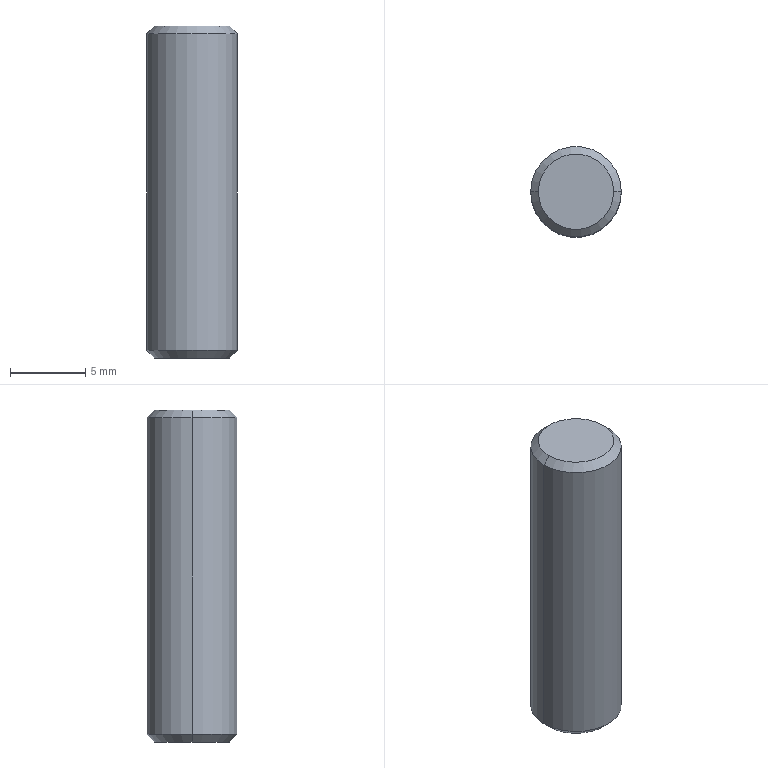Part | STEP file | 03-18 guide post A | 1 solid | 12 faces | box 6 x 6 x 22 mm | volume 567.268 mm3 | cone 6 | cylinder 4 | plane 2 | commonest cylinder face diameters 2.5 x2 6 x2
STEP:
#1=CARTESIAN_POINT('',(1.25,0.,10.));
#2=VERTEX_POINT('',#1);
#3=CARTESIAN_POINT('',(-1.25,0.,10.));
#4=VERTEX_POINT('',#3);
#5=CARTESIAN_POINT('',(0.,0.,10.));
#6=DIRECTION('',(0.,0.,-1.));
#7=DIRECTION('',(-1.,0.,0.));
#8=AXIS2_PLACEMENT_3D('',#5,#6,#7);
#9=CIRCLE('',#8,1.25);
#10=EDGE_CURVE('',#2,#4,#9,.T.);
#11=ORIENTED_EDGE('',*,*,#10,.F.);
#12=CARTESIAN_POINT('',(1.25,0.,0.));
#13=VERTEX_POINT('',#12);
#14=CARTESIAN_POINT('',(1.25,0.,0.));
#15=DIRECTION('',(0.,0.,-1.));
#16=VECTOR('',#15,1000.);
#17=LINE('',#14,#16);
#18=EDGE_CURVE('',#2,#13,#17,.T.);
#19=ORIENTED_EDGE('',*,*,#18,.T.);
#20=CARTESIAN_POINT('',(-1.25,0.,0.));
#21=VERTEX_POINT('',#20);
#22=CARTESIAN_POINT('',(0.,0.,0.));
#23=DIRECTION('',(0.,0.,-1.));
#24=DIRECTION('',(-1.,0.,0.));
#25=AXIS2_PLACEMENT_3D('',#22,#23,#24);
#26=CIRCLE('',#25,1.25);
#27=EDGE_CURVE('',#13,#21,#26,.T.);
#28=ORIENTED_EDGE('',*,*,#27,.T.);
#29=CARTESIAN_POINT('',(-1.25,0.,0.));
#30=DIRECTION('',(0.,0.,-1.));
#31=VECTOR('',#30,1000.);
#32=LINE('',#29,#31);
#33=EDGE_CURVE('',#4,#21,#32,.T.);
#34=ORIENTED_EDGE('',*,*,#33,.F.);
#35=EDGE_LOOP('',(#11,#19,#28,#34));
#36=FACE_OUTER_BOUND('',#35,.T.);
#37=CARTESIAN_POINT('',(0.,0.,0.));
#38=DIRECTION('',(0.,0.,-1.));
#39=DIRECTION('',(-1.,0.,0.));
#40=AXIS2_PLACEMENT_3D('',#37,#38,#39);
#41=CYLINDRICAL_SURFACE('',#40,1.25);
#42=ADVANCED_FACE('',(#36),#41,.F.);
#43=CARTESIAN_POINT('',(0.,0.,10.751));
#44=VERTEX_POINT('',#43);
#45=CARTESIAN_POINT('',(-1.25,0.,10.));
#46=DIRECTION('',(-0.8572,0.,-0.515));
#47=VECTOR('',#46,1000.);
#48=LINE('',#45,#47);
#49=EDGE_CURVE('',#44,#4,#48,.T.);
#50=ORIENTED_EDGE('',*,*,#49,.F.);
#51=CARTESIAN_POINT('',(1.25,0.,10.));
#52=DIRECTION('',(0.8572,0.,-0.515));
#53=VECTOR('',#52,1000.);
#54=LINE('',#51,#53);
#55=EDGE_CURVE('',#44,#2,#54,.T.);
#56=ORIENTED_EDGE('',*,*,#55,.T.);
#57=ORIENTED_EDGE('',*,*,#10,.T.);
#58=EDGE_LOOP('',(#50,#56,#57));
#59=FACE_OUTER_BOUND('',#58,.T.);
#60=CARTESIAN_POINT('',(0.,0.,10.));
#61=DIRECTION('',(0.,0.,-1.));
#62=DIRECTION('',(-1.,0.,0.));
#63=AXIS2_PLACEMENT_3D('',#60,#61,#62);
#64=CONICAL_SURFACE('',#63,1.25,1.03);
#65=ADVANCED_FACE('',(#59),#64,.F.);
#66=CARTESIAN_POINT('',(-2.5,0.,0.));
#67=VERTEX_POINT('',#66);
#68=CARTESIAN_POINT('',(2.5,0.,0.));
#69=VERTEX_POINT('',#68);
#70=CARTESIAN_POINT('',(0.,0.,0.));
#71=DIRECTION('',(0.,0.,-1.));
#72=DIRECTION('',(1.,0.,0.));
#73=AXIS2_PLACEMENT_3D('',#70,#71,#72);
#74=CIRCLE('',#73,2.5);
#75=EDGE_CURVE('',#67,#69,#74,.T.);
#76=ORIENTED_EDGE('',*,*,#75,.F.);
#77=CARTESIAN_POINT('',(-3.,0.,0.5));
#78=VERTEX_POINT('',#77);
#79=CARTESIAN_POINT('',(-3.,0.,0.5));
#80=DIRECTION('',(-0.7071,0.,0.7071));
#81=VECTOR('',#80,1000.);
#82=LINE('',#79,#81);
#83=EDGE_CURVE('',#67,#78,#82,.T.);
#84=ORIENTED_EDGE('',*,*,#83,.T.);
#85=CARTESIAN_POINT('',(3.,0.,0.5));
#86=VERTEX_POINT('',#85);
#87=CARTESIAN_POINT('',(0.,0.,0.5));
#88=DIRECTION('',(0.,0.,1.));
#89=DIRECTION('',(1.,0.,0.));
#90=AXIS2_PLACEMENT_3D('',#87,#88,#89);
#91=CIRCLE('',#90,3.);
#92=EDGE_CURVE('',#86,#78,#91,.T.);
#93=ORIENTED_EDGE('',*,*,#92,.F.);
#94=CARTESIAN_POINT('',(3.,0.,0.5));
#95=DIRECTION('',(0.7071,0.,0.7071));
#96=VECTOR('',#95,1000.);
#97=LINE('',#94,#96);
#98=EDGE_CURVE('',#69,#86,#97,.T.);
#99=ORIENTED_EDGE('',*,*,#98,.F.);
#100=EDGE_LOOP('',(#76,#84,#93,#99));
#101=FACE_OUTER_BOUND('',#100,.T.);
#102=CARTESIAN_POINT('',(0.,0.,0.5));
#103=DIRECTION('',(0.,0.,1.));
#104=DIRECTION('',(1.,0.,0.));
#105=AXIS2_PLACEMENT_3D('',#102,#103,#104);
#106=CONICAL_SURFACE('',#105,3.,0.7854);
#107=ADVANCED_FACE('',(#101),#106,.T.);
#108=CARTESIAN_POINT('',(2.5,0.,22.));
#109=VERTEX_POINT('',#108);
#110=CARTESIAN_POINT('',(-2.5,0.,22.));
#111=VERTEX_POINT('',#110);
#112=CARTESIAN_POINT('',(0.,0.,22.));
#113=DIRECTION('',(0.,0.,1.));
#114=DIRECTION('',(1.,0.,0.));
#115=AXIS2_PLACEMENT_3D('',#112,#113,#114);
#116=CIRCLE('',#115,2.5);
#117=EDGE_CURVE('',#109,#111,#116,.T.);
#118=ORIENTED_EDGE('',*,*,#117,.F.);
#119=CARTESIAN_POINT('',(3.,0.,21.5));
#120=VERTEX_POINT('',#119);
#121=CARTESIAN_POINT('',(2.5,0.,22.));
#122=DIRECTION('',(0.7071,0.,-0.7071));
#123=VECTOR('',#122,1000.);
#124=LINE('',#121,#123);
#125=EDGE_CURVE('',#109,#120,#124,.T.);
#126=ORIENTED_EDGE('',*,*,#125,.T.);
#127=CARTESIAN_POINT('',(-3.,0.,21.5));
#128=VERTEX_POINT('',#127);
#129=CARTESIAN_POINT('',(0.,0.,21.5));
#130=DIRECTION('',(0.,0.,-1.));
#131=DIRECTION('',(1.,0.,0.));
#132=AXIS2_PLACEMENT_3D('',#129,#130,#131);
#133=CIRCLE('',#132,3.);
#134=EDGE_CURVE('',#128,#120,#133,.T.);
#135=ORIENTED_EDGE('',*,*,#134,.F.);
#136=CARTESIAN_POINT('',(-2.5,0.,22.));
#137=DIRECTION('',(-0.7071,0.,-0.7071));
#138=VECTOR('',#137,1000.);
#139=LINE('',#136,#138);
#140=EDGE_CURVE('',#111,#128,#139,.T.);
#141=ORIENTED_EDGE('',*,*,#140,.F.);
#142=EDGE_LOOP('',(#118,#126,#135,#141));
#143=FACE_OUTER_BOUND('',#142,.T.);
#144=CARTESIAN_POINT('',(0.,0.,22.));
#145=DIRECTION('',(0.,0.,-1.));
#146=DIRECTION('',(-1.,0.,0.));
#147=AXIS2_PLACEMENT_3D('',#144,#145,#146);
#148=CONICAL_SURFACE('',#147,2.5,0.7854);
#149=ADVANCED_FACE('',(#143),#148,.T.);
#150=ORIENTED_EDGE('',*,*,#134,.T.);
#151=CARTESIAN_POINT('',(3.,0.,22.));
#152=DIRECTION('',(0.,0.,-1.));
#153=VECTOR('',#152,1000.);
#154=LINE('',#151,#153);
#155=EDGE_CURVE('',#120,#86,#154,.T.);
#156=ORIENTED_EDGE('',*,*,#155,.T.);
#157=ORIENTED_EDGE('',*,*,#92,.T.);
#158=CARTESIAN_POINT('',(-3.,0.,22.));
#159=DIRECTION('',(0.,0.,-1.));
#160=VECTOR('',#159,1000.);
#161=LINE('',#158,#160);
#162=EDGE_CURVE('',#128,#78,#161,.T.);
#163=ORIENTED_EDGE('',*,*,#162,.F.);
#164=EDGE_LOOP('',(#150,#156,#157,#163));
#165=FACE_OUTER_BOUND('',#164,.T.);
#166=CARTESIAN_POINT('',(0.,0.,22.));
#167=DIRECTION('',(0.,0.,-1.));
#168=DIRECTION('',(-1.,0.,0.));
#169=AXIS2_PLACEMENT_3D('',#166,#167,#168);
#170=CYLINDRICAL_SURFACE('',#169,3.);
#171=ADVANCED_FACE('',(#165),#170,.T.);
#172=ORIENTED_EDGE('',*,*,#155,.F.);
#173=CARTESIAN_POINT('',(0.,0.,21.5));
#174=DIRECTION('',(0.,0.,-1.));
#175=DIRECTION('',(1.,0.,0.));
#176=AXIS2_PLACEMENT_3D('',#173,#174,#175);
#177=CIRCLE('',#176,3.);
#178=EDGE_CURVE('',#120,#128,#177,.T.);
#179=ORIENTED_EDGE('',*,*,#178,.T.);
#180=ORIENTED_EDGE('',*,*,#162,.T.);
#181=CARTESIAN_POINT('',(0.,0.,0.5));
#182=DIRECTION('',(0.,0.,1.));
#183=DIRECTION('',(1.,0.,0.));
#184=AXIS2_PLACEMENT_3D('',#181,#182,#183);
#185=CIRCLE('',#184,3.);
#186=EDGE_CURVE('',#78,#86,#185,.T.);
#187=ORIENTED_EDGE('',*,*,#186,.T.);
#188=EDGE_LOOP('',(#172,#179,#180,#187));
#189=FACE_OUTER_BOUND('',#188,.T.);
#190=CARTESIAN_POINT('',(0.,0.,22.));
#191=DIRECTION('',(0.,0.,-1.));
#192=DIRECTION('',(-1.,0.,0.));
#193=AXIS2_PLACEMENT_3D('',#190,#191,#192);
#194=CYLINDRICAL_SURFACE('',#193,3.);
#195=ADVANCED_FACE('',(#189),#194,.T.);
#196=CARTESIAN_POINT('',(0.,0.,22.));
#197=DIRECTION('',(0.,0.,1.));
#198=DIRECTION('',(1.,0.,0.));
#199=AXIS2_PLACEMENT_3D('',#196,#197,#198);
#200=CIRCLE('',#199,2.5);
#201=EDGE_CURVE('',#111,#109,#200,.T.);
#202=ORIENTED_EDGE('',*,*,#201,.T.);
#203=ORIENTED_EDGE('',*,*,#117,.T.);
#204=EDGE_LOOP('',(#202,#203));
#205=FACE_OUTER_BOUND('',#204,.T.);
#206=CARTESIAN_POINT('',(0.,0.,22.));
#207=DIRECTION('',(0.,0.,1.));
#208=DIRECTION('',(1.,0.,0.));
#209=AXIS2_PLACEMENT_3D('',#206,#207,#208);
#210=PLANE('',#209);
#211=ADVANCED_FACE('',(#205),#210,.T.);
#212=CARTESIAN_POINT('',(0.,0.,0.));
#213=DIRECTION('',(0.,0.,-1.));
#214=DIRECTION('',(-1.,0.,0.));
#215=AXIS2_PLACEMENT_3D('',#212,#213,#214);
#216=CIRCLE('',#215,1.25);
#217=EDGE_CURVE('',#21,#13,#216,.T.);
#218=ORIENTED_EDGE('',*,*,#217,.F.);
#219=ORIENTED_EDGE('',*,*,#27,.F.);
#220=EDGE_LOOP('',(#218,#219));
#221=FACE_BOUND('',#220,.T.);
#222=CARTESIAN_POINT('',(0.,0.,0.));
#223=DIRECTION('',(0.,0.,-1.));
#224=DIRECTION('',(1.,0.,0.));
#225=AXIS2_PLACEMENT_3D('',#222,#223,#224);
#226=CIRCLE('',#225,2.5);
#227=EDGE_CURVE('',#69,#67,#226,.T.);
#228=ORIENTED_EDGE('',*,*,#227,.T.);
#229=ORIENTED_EDGE('',*,*,#75,.T.);
#230=EDGE_LOOP('',(#228,#229));
#231=FACE_OUTER_BOUND('',#230,.T.);
#232=CARTESIAN_POINT('',(0.,0.,0.));
#233=DIRECTION('',(0.,0.,1.));
#234=DIRECTION('',(1.,0.,0.));
#235=AXIS2_PLACEMENT_3D('',#232,#233,#234);
#236=PLANE('',#235);
#237=ADVANCED_FACE('',(#221,#231),#236,.F.);
#238=ORIENTED_EDGE('',*,*,#125,.F.);
#239=ORIENTED_EDGE('',*,*,#201,.F.);
#240=ORIENTED_EDGE('',*,*,#140,.T.);
#241=ORIENTED_EDGE('',*,*,#178,.F.);
#242=EDGE_LOOP('',(#238,#239,#240,#241));
#243=FACE_OUTER_BOUND('',#242,.T.);
#244=CARTESIAN_POINT('',(0.,0.,22.));
#245=DIRECTION('',(0.,0.,-1.));
#246=DIRECTION('',(-1.,0.,0.));
#247=AXIS2_PLACEMENT_3D('',#244,#245,#246);
#248=CONICAL_SURFACE('',#247,2.5,0.7854);
#249=ADVANCED_FACE('',(#243),#248,.T.);
#250=ORIENTED_EDGE('',*,*,#83,.F.);
#251=ORIENTED_EDGE('',*,*,#227,.F.);
#252=ORIENTED_EDGE('',*,*,#98,.T.);
#253=ORIENTED_EDGE('',*,*,#186,.F.);
#254=EDGE_LOOP('',(#250,#251,#252,#253));
#255=FACE_OUTER_BOUND('',#254,.T.);
#256=CARTESIAN_POINT('',(0.,0.,0.5));
#257=DIRECTION('',(0.,0.,1.));
#258=DIRECTION('',(1.,0.,0.));
#259=AXIS2_PLACEMENT_3D('',#256,#257,#258);
#260=CONICAL_SURFACE('',#259,3.,0.7854);
#261=ADVANCED_FACE('',(#255),#260,.T.);
#262=ORIENTED_EDGE('',*,*,#55,.F.);
#263=ORIENTED_EDGE('',*,*,#49,.T.);
#264=CARTESIAN_POINT('',(0.,0.,10.));
#265=DIRECTION('',(0.,0.,-1.));
#266=DIRECTION('',(-1.,0.,0.));
#267=AXIS2_PLACEMENT_3D('',#264,#265,#266);
#268=CIRCLE('',#267,1.25);
#269=EDGE_CURVE('',#4,#2,#268,.T.);
#270=ORIENTED_EDGE('',*,*,#269,.T.);
#271=EDGE_LOOP('',(#262,#263,#270));
#272=FACE_OUTER_BOUND('',#271,.T.);
#273=CARTESIAN_POINT('',(0.,0.,10.));
#274=DIRECTION('',(0.,0.,-1.));
#275=DIRECTION('',(-1.,0.,0.));
#276=AXIS2_PLACEMENT_3D('',#273,#274,#275);
#277=CONICAL_SURFACE('',#276,1.25,1.03);
#278=ADVANCED_FACE('',(#272),#277,.F.);
#279=ORIENTED_EDGE('',*,*,#18,.F.);
#280=ORIENTED_EDGE('',*,*,#269,.F.);
#281=ORIENTED_EDGE('',*,*,#33,.T.);
#282=ORIENTED_EDGE('',*,*,#217,.T.);
#283=EDGE_LOOP('',(#279,#280,#281,#282));
#284=FACE_OUTER_BOUND('',#283,.T.);
#285=CARTESIAN_POINT('',(0.,0.,0.));
#286=DIRECTION('',(0.,0.,-1.));
#287=DIRECTION('',(-1.,0.,0.));
#288=AXIS2_PLACEMENT_3D('',#285,#286,#287);
#289=CYLINDRICAL_SURFACE('',#288,1.25);
#290=ADVANCED_FACE('',(#284),#289,.F.);
#291=CLOSED_SHELL('',(#42,#65,#107,#149,#171,#195,#211,#237,#249,#261,#278,#290));
#292=MANIFOLD_SOLID_BREP('',#291);
#293=CARTESIAN_POINT('',(0.,0.,0.));
#294=DIRECTION('',(0.,0.,1.));
#295=DIRECTION('',(1.,0.,0.));
#296=AXIS2_PLACEMENT_3D('',#293,#294,#295);
#297=(LENGTH_UNIT()NAMED_UNIT(*)SI_UNIT(.MILLI.,.METRE.));
#298=UNCERTAINTY_MEASURE_WITH_UNIT(LENGTH_MEASURE(0.00001),#297,'','');
#299=(NAMED_UNIT(*)PLANE_ANGLE_UNIT()SI_UNIT($,.RADIAN.));
#300=(NAMED_UNIT(*)SI_UNIT($,.STERADIAN.)SOLID_ANGLE_UNIT());
#301=(GEOMETRIC_REPRESENTATION_CONTEXT(3)GLOBAL_UNCERTAINTY_ASSIGNED_CONTEXT((#298))GLOBAL_UNIT_ASSIGNED_CONTEXT((#297,#299,#300))REPRESENTATION_CONTEXT('',''));
#302=ADVANCED_BREP_SHAPE_REPRESENTATION('',(#292,#296),#301);